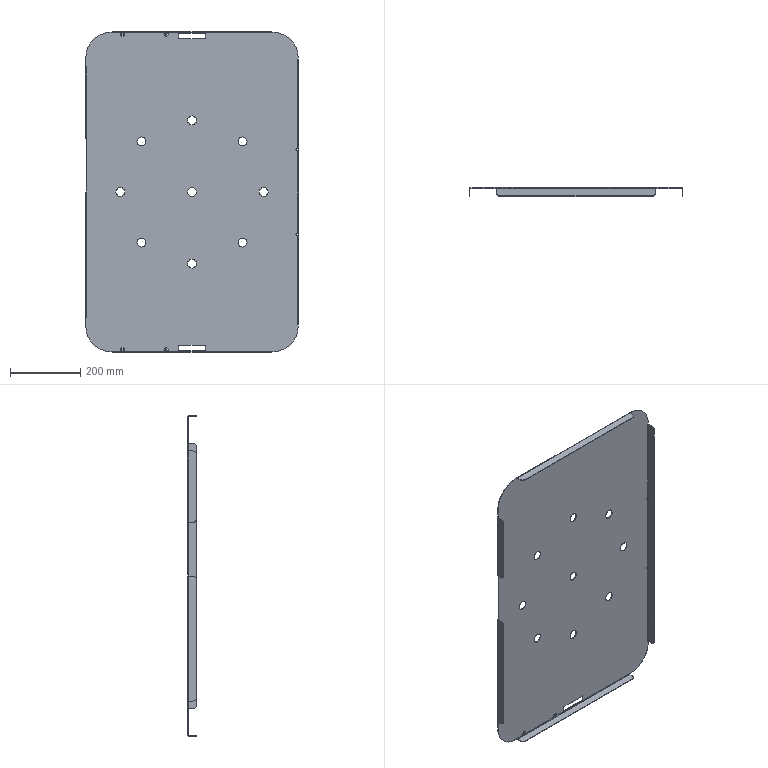Part | NX | features BREP 1 | 1 solid | 164 faces | box 606.247 x 24.003 x 910.285 mm | volume 878435 mm3 | plane 86 | cylinder 66 | spline 12 | commonest cylinder face diameters 25.4 x18 19.05 x10 10.998 x8 3.175 x7 6.172 x7 1.587 x4